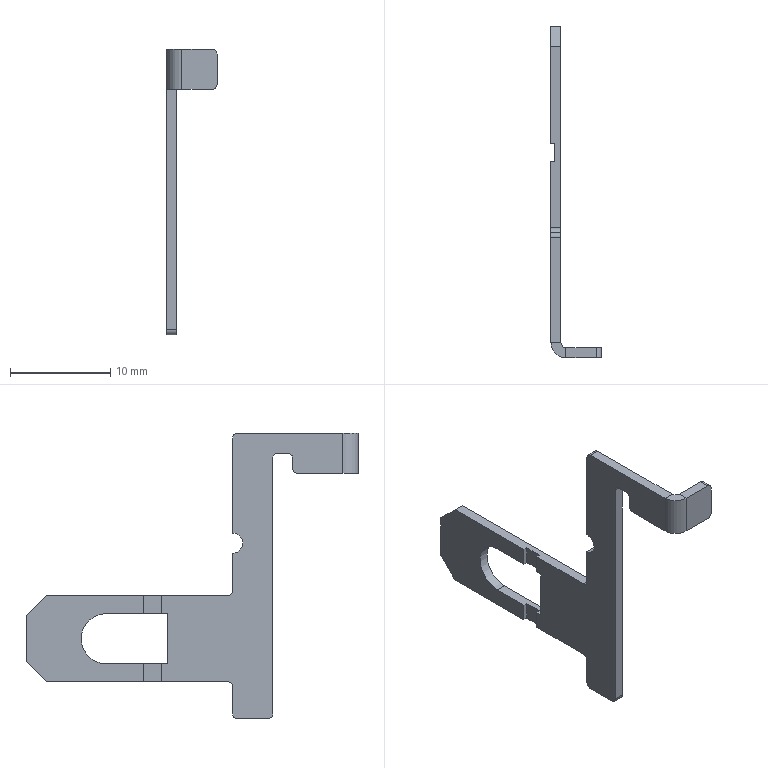Part | SolidWorks | features ICE 6, FlatPattern 2, Chamfer 1, Fillet 1, MirrorSolid 1, SMBaseFlange 1, SheetMetal 1 | 1 solid | 47 faces | box 5 x 33.1 x 28.5 mm | volume 286.856 mm3 | plane 33 | cylinder 14 | commonest cylinder face diameters 1 x11 2 x1 3 x1 5 x1
STEP:
#1=CARTESIAN_POINT('',(-4.,12.5,67.02));
#2=VERTEX_POINT('',#1);
#3=CARTESIAN_POINT('',(-5.,12.5,67.02));
#4=VERTEX_POINT('',#3);
#5=CARTESIAN_POINT('',(0.,12.5,67.02));
#6=DIRECTION('',(-1.,0.,0.));
#7=VECTOR('',#6,1000.);
#8=LINE('',#5,#7);
#9=EDGE_CURVE('',#2,#4,#8,.T.);
#10=ORIENTED_EDGE('',*,*,#9,.T.);
#11=CARTESIAN_POINT('',(-5.,12.5,76.5));
#12=VERTEX_POINT('',#11);
#13=CARTESIAN_POINT('',(-5.,12.5,73.));
#14=DIRECTION('',(0.,0.,1.));
#15=VECTOR('',#14,1000.);
#16=LINE('',#13,#15);
#17=EDGE_CURVE('',#4,#12,#16,.T.);
#18=ORIENTED_EDGE('',*,*,#17,.T.);
#19=CARTESIAN_POINT('',(-4.,12.5,76.5));
#20=VERTEX_POINT('',#19);
#21=CARTESIAN_POINT('',(-5.,12.5,76.5));
#22=DIRECTION('',(-1.,0.,0.));
#23=VECTOR('',#22,1000.);
#24=LINE('',#21,#23);
#25=EDGE_CURVE('',#20,#12,#24,.T.);
#26=ORIENTED_EDGE('',*,*,#25,.F.);
#27=CARTESIAN_POINT('',(-4.,12.5,73.));
#28=DIRECTION('',(0.,0.,1.));
#29=VECTOR('',#28,1000.);
#30=LINE('',#27,#29);
#31=EDGE_CURVE('',#2,#20,#30,.T.);
#32=ORIENTED_EDGE('',*,*,#31,.F.);
#33=EDGE_LOOP('',(#10,#18,#26,#32));
#34=FACE_OUTER_BOUND('',#33,.T.);
#35=CARTESIAN_POINT('',(-5.,12.5,73.));
#36=DIRECTION('',(0.,1.,0.));
#37=DIRECTION('',(0.,0.,-1.));
#38=AXIS2_PLACEMENT_3D('',#35,#36,#37);
#39=PLANE('',#38);
#40=ADVANCED_FACE('',(#34),#39,.T.);
#41=CARTESIAN_POINT('',(-5.,21.4,54.));
#42=VERTEX_POINT('',#41);
#43=CARTESIAN_POINT('',(-5.,21.4,52.2));
#44=VERTEX_POINT('',#43);
#45=CARTESIAN_POINT('',(-5.,21.4,77.));
#46=DIRECTION('',(0.,0.,-1.));
#47=VECTOR('',#46,1000.);
#48=LINE('',#45,#47);
#49=EDGE_CURVE('',#42,#44,#48,.T.);
#50=ORIENTED_EDGE('',*,*,#49,.T.);
#51=CARTESIAN_POINT('',(-4.6,21.4,52.2));
#52=VERTEX_POINT('',#51);
#53=CARTESIAN_POINT('',(-5.,21.4,52.2));
#54=DIRECTION('',(-1.,0.,0.));
#55=VECTOR('',#54,1000.);
#56=LINE('',#53,#55);
#57=EDGE_CURVE('',#52,#44,#56,.T.);
#58=ORIENTED_EDGE('',*,*,#57,.F.);
#59=CARTESIAN_POINT('',(-4.6,21.4,54.));
#60=VERTEX_POINT('',#59);
#61=CARTESIAN_POINT('',(-4.6,21.4,77.));
#62=DIRECTION('',(0.,0.,-1.));
#63=VECTOR('',#62,1000.);
#64=LINE('',#61,#63);
#65=EDGE_CURVE('',#60,#52,#64,.T.);
#66=ORIENTED_EDGE('',*,*,#65,.F.);
#67=CARTESIAN_POINT('',(-5.,21.4,54.));
#68=DIRECTION('',(1.,0.,0.));
#69=VECTOR('',#68,1000.);
#70=LINE('',#67,#69);
#71=EDGE_CURVE('',#42,#60,#70,.T.);
#72=ORIENTED_EDGE('',*,*,#71,.F.);
#73=EDGE_LOOP('',(#50,#58,#66,#72));
#74=FACE_OUTER_BOUND('',#73,.T.);
#75=CARTESIAN_POINT('',(-5.,21.4,77.));
#76=DIRECTION('',(0.,1.,0.));
#77=DIRECTION('',(-1.,0.,0.));
#78=AXIS2_PLACEMENT_3D('',#75,#76,#77);
#79=PLANE('',#78);
#80=ADVANCED_FACE('',(#74),#79,.F.);
#81=ORIENTED_EDGE('',*,*,#65,.T.);
#82=CARTESIAN_POINT('',(-4.6,19.6,52.2));
#83=VERTEX_POINT('',#82);
#84=CARTESIAN_POINT('',(-4.6,21.4,52.2));
#85=DIRECTION('',(0.,1.,0.));
#86=VECTOR('',#85,1000.);
#87=LINE('',#84,#86);
#88=EDGE_CURVE('',#83,#52,#87,.T.);
#89=ORIENTED_EDGE('',*,*,#88,.F.);
#90=CARTESIAN_POINT('',(-4.6,19.6,54.));
#91=VERTEX_POINT('',#90);
#92=CARTESIAN_POINT('',(-4.6,19.6,77.));
#93=DIRECTION('',(0.,0.,-1.));
#94=VECTOR('',#93,1000.);
#95=LINE('',#92,#94);
#96=EDGE_CURVE('',#91,#83,#95,.T.);
#97=ORIENTED_EDGE('',*,*,#96,.F.);
#98=CARTESIAN_POINT('',(-4.6,21.4,54.));
#99=DIRECTION('',(0.,-1.,0.));
#100=VECTOR('',#99,1000.);
#101=LINE('',#98,#100);
#102=EDGE_CURVE('',#60,#91,#101,.T.);
#103=ORIENTED_EDGE('',*,*,#102,.F.);
#104=EDGE_LOOP('',(#81,#89,#97,#103));
#105=FACE_OUTER_BOUND('',#104,.T.);
#106=CARTESIAN_POINT('',(-4.6,21.4,77.));
#107=DIRECTION('',(1.,0.,0.));
#108=DIRECTION('',(0.,1.,0.));
#109=AXIS2_PLACEMENT_3D('',#106,#107,#108);
#110=PLANE('',#109);
#111=ADVANCED_FACE('',(#105),#110,.F.);
#112=ORIENTED_EDGE('',*,*,#96,.T.);
#113=CARTESIAN_POINT('',(-5.,19.6,52.2));
#114=VERTEX_POINT('',#113);
#115=CARTESIAN_POINT('',(-5.,19.6,52.2));
#116=DIRECTION('',(1.,0.,0.));
#117=VECTOR('',#116,1000.);
#118=LINE('',#115,#117);
#119=EDGE_CURVE('',#114,#83,#118,.T.);
#120=ORIENTED_EDGE('',*,*,#119,.F.);
#121=CARTESIAN_POINT('',(-5.,19.6,54.));
#122=VERTEX_POINT('',#121);
#123=CARTESIAN_POINT('',(-5.,19.6,77.));
#124=DIRECTION('',(0.,0.,-1.));
#125=VECTOR('',#124,1000.);
#126=LINE('',#123,#125);
#127=EDGE_CURVE('',#122,#114,#126,.T.);
#128=ORIENTED_EDGE('',*,*,#127,.F.);
#129=CARTESIAN_POINT('',(-5.,19.6,54.));
#130=DIRECTION('',(-1.,0.,0.));
#131=VECTOR('',#130,1000.);
#132=LINE('',#129,#131);
#133=EDGE_CURVE('',#91,#122,#132,.T.);
#134=ORIENTED_EDGE('',*,*,#133,.F.);
#135=EDGE_LOOP('',(#112,#120,#128,#134));
#136=FACE_OUTER_BOUND('',#135,.T.);
#137=CARTESIAN_POINT('',(-5.,19.6,77.));
#138=DIRECTION('',(0.,-1.,0.));
#139=DIRECTION('',(0.,0.,1.));
#140=AXIS2_PLACEMENT_3D('',#137,#138,#139);
#141=PLANE('',#140);
#142=ADVANCED_FACE('',(#136),#141,.F.);
#143=CARTESIAN_POINT('',(-5.,31.1,52.2));
#144=VERTEX_POINT('',#143);
#145=CARTESIAN_POINT('',(-5.,12.5,52.2));
#146=DIRECTION('',(0.,1.,0.));
#147=VECTOR('',#146,1000.);
#148=LINE('',#145,#147);
#149=EDGE_CURVE('',#44,#144,#148,.T.);
#150=ORIENTED_EDGE('',*,*,#149,.F.);
#151=ORIENTED_EDGE('',*,*,#49,.F.);
#152=CARTESIAN_POINT('',(-5.,25.1,54.));
#153=VERTEX_POINT('',#152);
#154=CARTESIAN_POINT('',(-5.,25.1,54.));
#155=DIRECTION('',(0.,1.,0.));
#156=VECTOR('',#155,1000.);
#157=LINE('',#154,#156);
#158=EDGE_CURVE('',#42,#153,#157,.T.);
#159=ORIENTED_EDGE('',*,*,#158,.T.);
#160=CARTESIAN_POINT('',(-5.,25.1,59.));
#161=VERTEX_POINT('',#160);
#162=CARTESIAN_POINT('',(-5.,25.1,56.5));
#163=DIRECTION('',(1.,0.,0.));
#164=DIRECTION('',(0.,0.,-1.));
#165=AXIS2_PLACEMENT_3D('',#162,#163,#164);
#166=CIRCLE('',#165,2.5);
#167=EDGE_CURVE('',#153,#161,#166,.T.);
#168=ORIENTED_EDGE('',*,*,#167,.T.);
#169=CARTESIAN_POINT('',(-5.,21.4,59.));
#170=VERTEX_POINT('',#169);
#171=CARTESIAN_POINT('',(-5.,25.1,59.));
#172=DIRECTION('',(0.,-1.,0.));
#173=VECTOR('',#172,1000.);
#174=LINE('',#171,#173);
#175=EDGE_CURVE('',#161,#170,#174,.T.);
#176=ORIENTED_EDGE('',*,*,#175,.T.);
#177=CARTESIAN_POINT('',(-5.,21.4,60.8));
#178=VERTEX_POINT('',#177);
#179=CARTESIAN_POINT('',(-5.,21.4,77.));
#180=DIRECTION('',(0.,0.,-1.));
#181=VECTOR('',#180,1000.);
#182=LINE('',#179,#181);
#183=EDGE_CURVE('',#178,#170,#182,.T.);
#184=ORIENTED_EDGE('',*,*,#183,.F.);
#185=CARTESIAN_POINT('',(-5.,31.1,60.8));
#186=VERTEX_POINT('',#185);
#187=CARTESIAN_POINT('',(-5.,12.5,60.8));
#188=DIRECTION('',(0.,-1.,0.));
#189=VECTOR('',#188,1000.);
#190=LINE('',#187,#189);
#191=EDGE_CURVE('',#186,#178,#190,.T.);
#192=ORIENTED_EDGE('',*,*,#191,.F.);
#193=CARTESIAN_POINT('',(-5.,33.1,58.8));
#194=VERTEX_POINT('',#193);
#195=CARTESIAN_POINT('',(-5.,9.45,82.45));
#196=DIRECTION('',(0.,-0.7071,0.7071));
#197=VECTOR('',#196,1000.);
#198=LINE('',#195,#197);
#199=EDGE_CURVE('',#194,#186,#198,.T.);
#200=ORIENTED_EDGE('',*,*,#199,.F.);
#201=CARTESIAN_POINT('',(-5.,33.1,54.2));
#202=VERTEX_POINT('',#201);
#203=CARTESIAN_POINT('',(-5.,33.1,60.8));
#204=DIRECTION('',(0.,0.,1.));
#205=VECTOR('',#204,1000.);
#206=LINE('',#203,#205);
#207=EDGE_CURVE('',#202,#194,#206,.T.);
#208=ORIENTED_EDGE('',*,*,#207,.F.);
#209=CARTESIAN_POINT('',(-5.,25.95,47.05));
#210=DIRECTION('',(0.,0.7071,0.7071));
#211=VECTOR('',#210,1000.);
#212=LINE('',#209,#211);
#213=EDGE_CURVE('',#144,#202,#212,.T.);
#214=ORIENTED_EDGE('',*,*,#213,.F.);
#215=EDGE_LOOP('',(#150,#151,#159,#168,#176,#184,#192,#200,#208,#214));
#216=FACE_OUTER_BOUND('',#215,.T.);
#217=CARTESIAN_POINT('',(-5.,0.,73.));
#218=DIRECTION('',(-1.,0.,0.));
#219=DIRECTION('',(0.,0.,-1.));
#220=AXIS2_PLACEMENT_3D('',#217,#218,#219);
#221=PLANE('',#220);
#222=ADVANCED_FACE('',(#216),#221,.T.);
#223=CARTESIAN_POINT('',(-5.,12.5,49.));
#224=VERTEX_POINT('',#223);
#225=CARTESIAN_POINT('',(-5.,12.5,51.7));
#226=VERTEX_POINT('',#225);
#227=CARTESIAN_POINT('',(-5.,12.5,73.));
#228=DIRECTION('',(0.,0.,1.));
#229=VECTOR('',#228,1000.);
#230=LINE('',#227,#229);
#231=EDGE_CURVE('',#224,#226,#230,.T.);
#232=ORIENTED_EDGE('',*,*,#231,.T.);
#233=CARTESIAN_POINT('',(-4.,12.5,51.7));
#234=VERTEX_POINT('',#233);
#235=CARTESIAN_POINT('',(-5.,12.5,51.7));
#236=DIRECTION('',(-1.,0.,0.));
#237=VECTOR('',#236,1000.);
#238=LINE('',#235,#237);
#239=EDGE_CURVE('',#234,#226,#238,.T.);
#240=ORIENTED_EDGE('',*,*,#239,.F.);
#241=CARTESIAN_POINT('',(-4.,12.5,49.));
#242=VERTEX_POINT('',#241);
#243=CARTESIAN_POINT('',(-4.,12.5,73.));
#244=DIRECTION('',(0.,0.,1.));
#245=VECTOR('',#244,1000.);
#246=LINE('',#243,#245);
#247=EDGE_CURVE('',#242,#234,#246,.T.);
#248=ORIENTED_EDGE('',*,*,#247,.F.);
#249=CARTESIAN_POINT('',(-5.,12.5,49.));
#250=DIRECTION('',(1.,0.,0.));
#251=VECTOR('',#250,1000.);
#252=LINE('',#249,#251);
#253=EDGE_CURVE('',#224,#242,#252,.T.);
#254=ORIENTED_EDGE('',*,*,#253,.F.);
#255=EDGE_LOOP('',(#232,#240,#248,#254));
#256=FACE_OUTER_BOUND('',#255,.T.);
#257=CARTESIAN_POINT('',(-5.,12.5,73.));
#258=DIRECTION('',(0.,1.,0.));
#259=DIRECTION('',(0.,0.,-1.));
#260=AXIS2_PLACEMENT_3D('',#257,#258,#259);
#261=PLANE('',#260);
#262=ADVANCED_FACE('',(#256),#261,.T.);
#263=CARTESIAN_POINT('',(-4.,1.5,73.));
#264=VERTEX_POINT('',#263);
#265=CARTESIAN_POINT('',(-4.,6.,73.));
#266=VERTEX_POINT('',#265);
#267=CARTESIAN_POINT('',(-4.,0.,73.));
#268=DIRECTION('',(0.,1.,0.));
#269=VECTOR('',#268,1000.);
#270=LINE('',#267,#269);
#271=EDGE_CURVE('',#264,#266,#270,.T.);
#272=ORIENTED_EDGE('',*,*,#271,.F.);
#273=CARTESIAN_POINT('',(-5.,1.5,73.));
#274=VERTEX_POINT('',#273);
#275=CARTESIAN_POINT('',(-5.,1.5,73.));
#276=DIRECTION('',(1.,0.,0.));
#277=VECTOR('',#276,1000.);
#278=LINE('',#275,#277);
#279=EDGE_CURVE('',#274,#264,#278,.T.);
#280=ORIENTED_EDGE('',*,*,#279,.F.);
#281=CARTESIAN_POINT('',(-5.,6.,73.));
#282=VERTEX_POINT('',#281);
#283=CARTESIAN_POINT('',(-5.,0.,73.));
#284=DIRECTION('',(0.,1.,0.));
#285=VECTOR('',#284,1000.);
#286=LINE('',#283,#285);
#287=EDGE_CURVE('',#274,#282,#286,.T.);
#288=ORIENTED_EDGE('',*,*,#287,.T.);
#289=CARTESIAN_POINT('',(-5.,6.,73.));
#290=DIRECTION('',(-1.,0.,0.));
#291=VECTOR('',#290,1000.);
#292=LINE('',#289,#291);
#293=EDGE_CURVE('',#266,#282,#292,.T.);
#294=ORIENTED_EDGE('',*,*,#293,.F.);
#295=EDGE_LOOP('',(#272,#280,#288,#294));
#296=FACE_OUTER_BOUND('',#295,.T.);
#297=CARTESIAN_POINT('',(-3.5,1.,73.));
#298=DIRECTION('',(0.,0.,-1.));
#299=DIRECTION('',(1.,0.,0.));
#300=AXIS2_PLACEMENT_3D('',#297,#298,#299);
#301=PLANE('',#300);
#302=ADVANCED_FACE('',(#296),#301,.T.);
#303=ORIENTED_EDGE('',*,*,#279,.T.);
#304=CARTESIAN_POINT('',(-3.5,1.,73.));
#305=VERTEX_POINT('',#304);
#306=CARTESIAN_POINT('',(-3.5,1.5,73.));
#307=DIRECTION('',(0.,0.,-1.));
#308=DIRECTION('',(1.,0.,0.));
#309=AXIS2_PLACEMENT_3D('',#306,#307,#308);
#310=CIRCLE('',#309,0.5);
#311=EDGE_CURVE('',#305,#264,#310,.T.);
#312=ORIENTED_EDGE('',*,*,#311,.F.);
#313=CARTESIAN_POINT('',(-3.5,0.,73.));
#314=VERTEX_POINT('',#313);
#315=CARTESIAN_POINT('',(-3.5,1.,73.));
#316=DIRECTION('',(0.,-1.,0.));
#317=VECTOR('',#316,1000.);
#318=LINE('',#315,#317);
#319=EDGE_CURVE('',#305,#314,#318,.T.);
#320=ORIENTED_EDGE('',*,*,#319,.T.);
#321=CARTESIAN_POINT('',(-3.5,1.5,73.));
#322=DIRECTION('',(0.,0.,-1.));
#323=DIRECTION('',(1.,0.,0.));
#324=AXIS2_PLACEMENT_3D('',#321,#322,#323);
#325=CIRCLE('',#324,1.5);
#326=EDGE_CURVE('',#314,#274,#325,.T.);
#327=ORIENTED_EDGE('',*,*,#326,.T.);
#328=EDGE_LOOP('',(#303,#312,#320,#327));
#329=FACE_OUTER_BOUND('',#328,.T.);
#330=CARTESIAN_POINT('',(-5.,1.5,73.));
#331=DIRECTION('',(0.,0.,-1.));
#332=DIRECTION('',(1.,0.,0.));
#333=AXIS2_PLACEMENT_3D('',#330,#331,#332);
#334=PLANE('',#333);
#335=ADVANCED_FACE('',(#329),#334,.T.);
#336=CARTESIAN_POINT('',(-3.5,0.,77.));
#337=VERTEX_POINT('',#336);
#338=CARTESIAN_POINT('',(-3.5,1.,77.));
#339=VERTEX_POINT('',#338);
#340=CARTESIAN_POINT('',(-3.5,0.,77.));
#341=DIRECTION('',(0.,1.,0.));
#342=VECTOR('',#341,1000.);
#343=LINE('',#340,#342);
#344=EDGE_CURVE('',#337,#339,#343,.T.);
#345=ORIENTED_EDGE('',*,*,#344,.T.);
#346=CARTESIAN_POINT('',(-4.,1.5,77.));
#347=VERTEX_POINT('',#346);
#348=CARTESIAN_POINT('',(-3.5,1.5,77.));
#349=DIRECTION('',(0.,0.,-1.));
#350=DIRECTION('',(1.,0.,0.));
#351=AXIS2_PLACEMENT_3D('',#348,#349,#350);
#352=CIRCLE('',#351,0.5);
#353=EDGE_CURVE('',#339,#347,#352,.T.);
#354=ORIENTED_EDGE('',*,*,#353,.T.);
#355=CARTESIAN_POINT('',(-5.,1.5,77.));
#356=VERTEX_POINT('',#355);
#357=CARTESIAN_POINT('',(-4.,1.5,77.));
#358=DIRECTION('',(-1.,0.,0.));
#359=VECTOR('',#358,1000.);
#360=LINE('',#357,#359);
#361=EDGE_CURVE('',#347,#356,#360,.T.);
#362=ORIENTED_EDGE('',*,*,#361,.T.);
#363=CARTESIAN_POINT('',(-3.5,1.5,77.));
#364=DIRECTION('',(0.,0.,-1.));
#365=DIRECTION('',(1.,0.,0.));
#366=AXIS2_PLACEMENT_3D('',#363,#364,#365);
#367=CIRCLE('',#366,1.5);
#368=EDGE_CURVE('',#337,#356,#367,.T.);
#369=ORIENTED_EDGE('',*,*,#368,.F.);
#370=EDGE_LOOP('',(#345,#354,#362,#369));
#371=FACE_OUTER_BOUND('',#370,.T.);
#372=CARTESIAN_POINT('',(-3.5,0.,77.));
#373=DIRECTION('',(0.,0.,1.));
#374=DIRECTION('',(-1.,0.,0.));
#375=AXIS2_PLACEMENT_3D('',#372,#373,#374);
#376=PLANE('',#375);
#377=ADVANCED_FACE('',(#371),#376,.T.);
#378=CARTESIAN_POINT('',(-0.5,1.,77.));
#379=VERTEX_POINT('',#378);
#380=CARTESIAN_POINT('',(0.,1.,77.));
#381=DIRECTION('',(-1.,0.,0.));
#382=VECTOR('',#381,1000.);
#383=LINE('',#380,#382);
#384=EDGE_CURVE('',#379,#339,#383,.T.);
#385=ORIENTED_EDGE('',*,*,#384,.T.);
#386=ORIENTED_EDGE('',*,*,#344,.F.);
#387=CARTESIAN_POINT('',(-0.5,0.,77.));
#388=VERTEX_POINT('',#387);
#389=CARTESIAN_POINT('',(0.,0.,77.));
#390=DIRECTION('',(-1.,0.,0.));
#391=VECTOR('',#390,1000.);
#392=LINE('',#389,#391);
#393=EDGE_CURVE('',#388,#337,#392,.T.);
#394=ORIENTED_EDGE('',*,*,#393,.F.);
#395=CARTESIAN_POINT('',(-0.5,1.5,77.));
#396=DIRECTION('',(0.,-1.,0.));
#397=VECTOR('',#396,1000.);
#398=LINE('',#395,#397);
#399=EDGE_CURVE('',#379,#388,#398,.T.);
#400=ORIENTED_EDGE('',*,*,#399,.F.);
#401=EDGE_LOOP('',(#385,#386,#394,#400));
#402=FACE_OUTER_BOUND('',#401,.T.);
#403=CARTESIAN_POINT('',(-4.,1.5,77.));
#404=DIRECTION('',(0.,0.,1.));
#405=DIRECTION('',(-1.,0.,0.));
#406=AXIS2_PLACEMENT_3D('',#403,#404,#405);
#407=PLANE('',#406);
#408=ADVANCED_FACE('',(#402),#407,.T.);
#409=CARTESIAN_POINT('',(-4.,19.,54.));
#410=VERTEX_POINT('',#409);
#411=CARTESIAN_POINT('',(-4.,25.1,54.));
#412=VERTEX_POINT('',#411);
#413=CARTESIAN_POINT('',(-4.,0.,54.));
#414=DIRECTION('',(0.,1.,0.));
#415=VECTOR('',#414,1000.);
#416=LINE('',#413,#415);
#417=EDGE_CURVE('',#410,#412,#416,.T.);
#418=ORIENTED_EDGE('',*,*,#417,.F.);
#419=CARTESIAN_POINT('',(-4.,19.,59.));
#420=VERTEX_POINT('',#419);
#421=CARTESIAN_POINT('',(-4.,19.,73.));
#422=DIRECTION('',(0.,0.,-1.));
#423=VECTOR('',#422,1000.);
#424=LINE('',#421,#423);
#425=EDGE_CURVE('',#420,#410,#424,.T.);
#426=ORIENTED_EDGE('',*,*,#425,.F.);
#427=CARTESIAN_POINT('',(-4.,25.1,59.));
#428=VERTEX_POINT('',#427);
#429=CARTESIAN_POINT('',(-4.,0.,59.));
#430=DIRECTION('',(0.,-1.,0.));
#431=VECTOR('',#430,1000.);
#432=LINE('',#429,#431);
#433=EDGE_CURVE('',#428,#420,#432,.T.);
#434=ORIENTED_EDGE('',*,*,#433,.F.);
#435=CARTESIAN_POINT('',(-4.,25.1,56.5));
#436=DIRECTION('',(1.,0.,0.));
#437=DIRECTION('',(0.,0.,-1.));
#438=AXIS2_PLACEMENT_3D('',#435,#436,#437);
#439=CIRCLE('',#438,2.5);
#440=EDGE_CURVE('',#412,#428,#439,.T.);
#441=ORIENTED_EDGE('',*,*,#440,.F.);
#442=EDGE_LOOP('',(#418,#426,#434,#441));
#443=FACE_BOUND('',#442,.T.);
#444=ORIENTED_EDGE('',*,*,#31,.T.);
#445=CARTESIAN_POINT('',(-4.,12.,77.));
#446=VERTEX_POINT('',#445);
#447=CARTESIAN_POINT('',(-4.,12.,76.5));
#448=DIRECTION('',(-1.,0.,0.));
#449=DIRECTION('',(0.,0.,-1.));
#450=AXIS2_PLACEMENT_3D('',#447,#448,#449);
#451=CIRCLE('',#450,0.5);
#452=EDGE_CURVE('',#446,#20,#451,.T.);
#453=ORIENTED_EDGE('',*,*,#452,.F.);
#454=CARTESIAN_POINT('',(-4.,0.,77.));
#455=DIRECTION('',(0.,1.,0.));
#456=VECTOR('',#455,1000.);
#457=LINE('',#454,#456);
#458=EDGE_CURVE('',#347,#446,#457,.T.);
#459=ORIENTED_EDGE('',*,*,#458,.F.);
#460=CARTESIAN_POINT('',(-4.,1.5,73.));
#461=DIRECTION('',(0.,0.,1.));
#462=VECTOR('',#461,1000.);
#463=LINE('',#460,#462);
#464=EDGE_CURVE('',#264,#347,#463,.T.);
#465=ORIENTED_EDGE('',*,*,#464,.F.);
#466=ORIENTED_EDGE('',*,*,#271,.T.);
#467=CARTESIAN_POINT('',(-4.,6.5,73.5));
#468=VERTEX_POINT('',#467);
#469=CARTESIAN_POINT('',(-4.,6.,73.5));
#470=DIRECTION('',(-1.,0.,0.));
#471=DIRECTION('',(0.,0.,-1.));
#472=AXIS2_PLACEMENT_3D('',#469,#470,#471);
#473=CIRCLE('',#472,0.5);
#474=EDGE_CURVE('',#468,#266,#473,.T.);
#475=ORIENTED_EDGE('',*,*,#474,.F.);
#476=CARTESIAN_POINT('',(-4.,6.5,74.5));
#477=VERTEX_POINT('',#476);
#478=CARTESIAN_POINT('',(-4.,6.5,73.));
#479=DIRECTION('',(0.,0.,-1.));
#480=VECTOR('',#479,1000.);
#481=LINE('',#478,#480);
#482=EDGE_CURVE('',#477,#468,#481,.T.);
#483=ORIENTED_EDGE('',*,*,#482,.F.);
#484=CARTESIAN_POINT('',(-4.,7.,75.));
#485=VERTEX_POINT('',#484);
#486=CARTESIAN_POINT('',(-4.,7.,74.5));
#487=DIRECTION('',(1.,0.,0.));
#488=DIRECTION('',(0.,0.,-1.));
#489=AXIS2_PLACEMENT_3D('',#486,#487,#488);
#490=CIRCLE('',#489,0.5);
#491=EDGE_CURVE('',#485,#477,#490,.T.);
#492=ORIENTED_EDGE('',*,*,#491,.F.);
#493=CARTESIAN_POINT('',(-4.,8.,75.));
#494=VERTEX_POINT('',#493);
#495=CARTESIAN_POINT('',(-4.,0.,75.));
#496=DIRECTION('',(0.,-1.,0.));
#497=VECTOR('',#496,1000.);
#498=LINE('',#495,#497);
#499=EDGE_CURVE('',#494,#485,#498,.T.);
#500=ORIENTED_EDGE('',*,*,#499,.F.);
#501=CARTESIAN_POINT('',(-4.,8.5,74.5));
#502=VERTEX_POINT('',#501);
#503=CARTESIAN_POINT('',(-4.,8.,74.5));
#504=DIRECTION('',(1.,0.,0.));
#505=DIRECTION('',(0.,0.,-1.));
#506=AXIS2_PLACEMENT_3D('',#503,#504,#505);
#507=CIRCLE('',#506,0.5);
#508=EDGE_CURVE('',#502,#494,#507,.T.);
#509=ORIENTED_EDGE('',*,*,#508,.F.);
#510=CARTESIAN_POINT('',(-4.,8.5,49.));
#511=VERTEX_POINT('',#510);
#512=CARTESIAN_POINT('',(-4.,8.5,73.));
#513=DIRECTION('',(0.,0.,1.));
#514=VECTOR('',#513,1000.);
#515=LINE('',#512,#514);
#516=EDGE_CURVE('',#511,#502,#515,.T.);
#517=ORIENTED_EDGE('',*,*,#516,.F.);
#518=CARTESIAN_POINT('',(-4.,9.,48.5));
#519=VERTEX_POINT('',#518);
#520=CARTESIAN_POINT('',(-4.,9.,49.));
#521=DIRECTION('',(-1.,0.,0.));
#522=DIRECTION('',(0.,0.,-1.));
#523=AXIS2_PLACEMENT_3D('',#520,#521,#522);
#524=CIRCLE('',#523,0.5);
#525=EDGE_CURVE('',#519,#511,#524,.T.);
#526=ORIENTED_EDGE('',*,*,#525,.F.);
#527=CARTESIAN_POINT('',(-4.,12.,48.5));
#528=VERTEX_POINT('',#527);
#529=CARTESIAN_POINT('',(-4.,8.5,48.5));
#530=DIRECTION('',(0.,1.,0.));
#531=VECTOR('',#530,1000.);
#532=LINE('',#529,#531);
#533=EDGE_CURVE('',#519,#528,#532,.T.);
#534=ORIENTED_EDGE('',*,*,#533,.T.);
#535=CARTESIAN_POINT('',(-4.,12.,49.));
#536=DIRECTION('',(-1.,0.,0.));
#537=DIRECTION('',(0.,0.,-1.));
#538=AXIS2_PLACEMENT_3D('',#535,#536,#537);
#539=CIRCLE('',#538,0.5);
#540=EDGE_CURVE('',#242,#528,#539,.T.);
#541=ORIENTED_EDGE('',*,*,#540,.F.);
#542=ORIENTED_EDGE('',*,*,#247,.T.);
#543=CARTESIAN_POINT('',(-4.,13.,52.2));
#544=VERTEX_POINT('',#543);
#545=CARTESIAN_POINT('',(-4.,13.,51.7));
#546=DIRECTION('',(1.,0.,0.));
#547=DIRECTION('',(0.,0.,-1.));
#548=AXIS2_PLACEMENT_3D('',#545,#546,#547);
#549=CIRCLE('',#548,0.5);
#550=EDGE_CURVE('',#544,#234,#549,.T.);
#551=ORIENTED_EDGE('',*,*,#550,.F.);
#552=CARTESIAN_POINT('',(-4.,31.1,52.2));
#553=VERTEX_POINT('',#552);
#554=CARTESIAN_POINT('',(-4.,12.5,52.2));
#555=DIRECTION('',(0.,-1.,0.));
#556=VECTOR('',#555,1000.);
#557=LINE('',#554,#556);
#558=EDGE_CURVE('',#553,#544,#557,.T.);
#559=ORIENTED_EDGE('',*,*,#558,.F.);
#560=CARTESIAN_POINT('',(-4.,33.1,54.2));
#561=VERTEX_POINT('',#560);
#562=CARTESIAN_POINT('',(-4.,31.1,52.2));
#563=DIRECTION('',(0.,-0.7071,-0.7071));
#564=VECTOR('',#563,1000.);
#565=LINE('',#562,#564);
#566=EDGE_CURVE('',#561,#553,#565,.T.);
#567=ORIENTED_EDGE('',*,*,#566,.F.);
#568=CARTESIAN_POINT('',(-4.,33.1,58.8));
#569=VERTEX_POINT('',#568);
#570=CARTESIAN_POINT('',(-4.,33.1,60.8));
#571=DIRECTION('',(0.,0.,-1.));
#572=VECTOR('',#571,1000.);
#573=LINE('',#570,#572);
#574=EDGE_CURVE('',#569,#561,#573,.T.);
#575=ORIENTED_EDGE('',*,*,#574,.F.);
#576=CARTESIAN_POINT('',(-4.,31.1,60.8));
#577=VERTEX_POINT('',#576);
#578=CARTESIAN_POINT('',(-4.,33.1,58.8));
#579=DIRECTION('',(0.,0.7071,-0.7071));
#580=VECTOR('',#579,1000.);
#581=LINE('',#578,#580);
#582=EDGE_CURVE('',#577,#569,#581,.T.);
#583=ORIENTED_EDGE('',*,*,#582,.F.);
#584=CARTESIAN_POINT('',(-4.,13.,60.8));
#585=VERTEX_POINT('',#584);
#586=CARTESIAN_POINT('',(-4.,12.5,60.8));
#587=DIRECTION('',(0.,1.,0.));
#588=VECTOR('',#587,1000.);
#589=LINE('',#586,#588);
#590=EDGE_CURVE('',#585,#577,#589,.T.);
#591=ORIENTED_EDGE('',*,*,#590,.F.);
#592=CARTESIAN_POINT('',(-4.,12.5,61.3));
#593=VERTEX_POINT('',#592);
#594=CARTESIAN_POINT('',(-4.,13.,61.3));
#595=DIRECTION('',(1.,0.,0.));
#596=DIRECTION('',(0.,0.,-1.));
#597=AXIS2_PLACEMENT_3D('',#594,#595,#596);
#598=CIRCLE('',#597,0.5);
#599=EDGE_CURVE('',#593,#585,#598,.T.);
#600=ORIENTED_EDGE('',*,*,#599,.F.);
#601=CARTESIAN_POINT('',(-4.,12.5,65.02));
#602=VERTEX_POINT('',#601);
#603=CARTESIAN_POINT('',(-4.,12.5,73.));
#604=DIRECTION('',(0.,0.,1.));
#605=VECTOR('',#604,1000.);
#606=LINE('',#603,#605);
#607=EDGE_CURVE('',#593,#602,#606,.T.);
#608=ORIENTED_EDGE('',*,*,#607,.T.);
#609=CARTESIAN_POINT('',(-4.,12.5,66.02));
#610=DIRECTION('',(1.,0.,0.));
#611=DIRECTION('',(0.,0.,-1.));
#612=AXIS2_PLACEMENT_3D('',#609,#610,#611);
#613=CIRCLE('',#612,1.);
#614=EDGE_CURVE('',#2,#602,#613,.T.);
#615=ORIENTED_EDGE('',*,*,#614,.F.);
#616=EDGE_LOOP('',(#444,#453,#459,#465,#466,#475,#483,#492,#500,#509,#517,#526,#534,#541,#542,#551,#559,#567,#575,#583,#591,#600,#608,#615));
#617=FACE_OUTER_BOUND('',#616,.T.);
#618=CARTESIAN_POINT('',(-4.,0.,73.));
#619=DIRECTION('',(-1.,0.,0.));
#620=DIRECTION('',(0.,0.,-1.));
#621=AXIS2_PLACEMENT_3D('',#618,#619,#620);
#622=PLANE('',#621);
#623=ADVANCED_FACE('',(#443,#617),#622,.F.);
#624=CARTESIAN_POINT('',(-5.,12.5,65.02));
#625=VERTEX_POINT('',#624);
#626=CARTESIAN_POINT('',(0.,12.5,65.02));
#627=DIRECTION('',(1.,0.,0.));
#628=VECTOR('',#627,1000.);
#629=LINE('',#626,#628);
#630=EDGE_CURVE('',#625,#602,#629,.T.);
#631=ORIENTED_EDGE('',*,*,#630,.T.);
#632=ORIENTED_EDGE('',*,*,#607,.F.);
#633=CARTESIAN_POINT('',(-5.,12.5,61.3));
#634=VERTEX_POINT('',#633);
#635=CARTESIAN_POINT('',(-4.,12.5,61.3));
#636=DIRECTION('',(1.,0.,0.));
#637=VECTOR('',#636,1000.);
#638=LINE('',#635,#637);
#639=EDGE_CURVE('',#634,#593,#638,.T.);
#640=ORIENTED_EDGE('',*,*,#639,.F.);
#641=CARTESIAN_POINT('',(-5.,12.5,73.));
#642=DIRECTION('',(0.,0.,1.));
#643=VECTOR('',#642,1000.);
#644=LINE('',#641,#643);
#645=EDGE_CURVE('',#634,#625,#644,.T.);
#646=ORIENTED_EDGE('',*,*,#645,.T.);
#647=EDGE_LOOP('',(#631,#632,#640,#646));
#648=FACE_OUTER_BOUND('',#647,.T.);
#649=CARTESIAN_POINT('',(-5.,12.5,73.));
#650=DIRECTION('',(0.,1.,0.));
#651=DIRECTION('',(0.,0.,-1.));
#652=AXIS2_PLACEMENT_3D('',#649,#650,#651);
#653=PLANE('',#652);
#654=ADVANCED_FACE('',(#648),#653,.T.);
#655=CARTESIAN_POINT('',(-5.,12.5,66.02));
#656=DIRECTION('',(1.,0.,0.));
#657=DIRECTION('',(0.,0.,-1.));
#658=AXIS2_PLACEMENT_3D('',#655,#656,#657);
#659=CIRCLE('',#658,1.);
#660=EDGE_CURVE('',#4,#625,#659,.T.);
#661=ORIENTED_EDGE('',*,*,#660,.T.);
#662=ORIENTED_EDGE('',*,*,#645,.F.);
#663=CARTESIAN_POINT('',(-5.,13.,60.8));
#664=VERTEX_POINT('',#663);
#665=CARTESIAN_POINT('',(-5.,13.,61.3));
#666=DIRECTION('',(-1.,0.,0.));
#667=DIRECTION('',(0.,0.,-1.));
#668=AXIS2_PLACEMENT_3D('',#665,#666,#667);
#669=CIRCLE('',#668,0.5);
#670=EDGE_CURVE('',#664,#634,#669,.T.);
#671=ORIENTED_EDGE('',*,*,#670,.F.);
#672=CARTESIAN_POINT('',(-5.,19.6,60.8));
#673=VERTEX_POINT('',#672);
#674=CARTESIAN_POINT('',(-5.,12.5,60.8));
#675=DIRECTION('',(0.,-1.,0.));
#676=VECTOR('',#675,1000.);
#677=LINE('',#674,#676);
#678=EDGE_CURVE('',#673,#664,#677,.T.);
#679=ORIENTED_EDGE('',*,*,#678,.F.);
#680=CARTESIAN_POINT('',(-5.,19.6,59.));
#681=VERTEX_POINT('',#680);
#682=CARTESIAN_POINT('',(-5.,19.6,77.));
#683=DIRECTION('',(0.,0.,-1.));
#684=VECTOR('',#683,1000.);
#685=LINE('',#682,#684);
#686=EDGE_CURVE('',#673,#681,#685,.T.);
#687=ORIENTED_EDGE('',*,*,#686,.T.);
#688=CARTESIAN_POINT('',(-5.,19.,59.));
#689=VERTEX_POINT('',#688);
#690=CARTESIAN_POINT('',(-5.,25.1,59.));
#691=DIRECTION('',(0.,-1.,0.));
#692=VECTOR('',#691,1000.);
#693=LINE('',#690,#692);
#694=EDGE_CURVE('',#681,#689,#693,.T.);
#695=ORIENTED_EDGE('',*,*,#694,.T.);
#696=CARTESIAN_POINT('',(-5.,19.,54.));
#697=VERTEX_POINT('',#696);
#698=CARTESIAN_POINT('',(-5.,19.,59.));
#699=DIRECTION('',(0.,0.,-1.));
#700=VECTOR('',#699,1000.);
#701=LINE('',#698,#700);
#702=EDGE_CURVE('',#689,#697,#701,.T.);
#703=ORIENTED_EDGE('',*,*,#702,.T.);
#704=CARTESIAN_POINT('',(-5.,25.1,54.));
#705=DIRECTION('',(0.,1.,0.));
#706=VECTOR('',#705,1000.);
#707=LINE('',#704,#706);
#708=EDGE_CURVE('',#697,#122,#707,.T.);
#709=ORIENTED_EDGE('',*,*,#708,.T.);
#710=ORIENTED_EDGE('',*,*,#127,.T.);
#711=CARTESIAN_POINT('',(-5.,13.,52.2));
#712=VERTEX_POINT('',#711);
#713=CARTESIAN_POINT('',(-5.,12.5,52.2));
#714=DIRECTION('',(0.,1.,0.));
#715=VECTOR('',#714,1000.);
#716=LINE('',#713,#715);
#717=EDGE_CURVE('',#712,#114,#716,.T.);
#718=ORIENTED_EDGE('',*,*,#717,.F.);
#719=CARTESIAN_POINT('',(-5.,13.,51.7));
#720=DIRECTION('',(-1.,0.,0.));
#721=DIRECTION('',(0.,0.,-1.));
#722=AXIS2_PLACEMENT_3D('',#719,#720,#721);
#723=CIRCLE('',#722,0.5);
#724=EDGE_CURVE('',#226,#712,#723,.T.);
#725=ORIENTED_EDGE('',*,*,#724,.F.);
#726=ORIENTED_EDGE('',*,*,#231,.F.);
#727=CARTESIAN_POINT('',(-5.,12.,48.5));
#728=VERTEX_POINT('',#727);
#729=CARTESIAN_POINT('',(-5.,12.,49.));
#730=DIRECTION('',(1.,0.,0.));
#731=DIRECTION('',(0.,0.,-1.));
#732=AXIS2_PLACEMENT_3D('',#729,#730,#731);
#733=CIRCLE('',#732,0.5);
#734=EDGE_CURVE('',#728,#224,#733,.T.);
#735=ORIENTED_EDGE('',*,*,#734,.F.);
#736=CARTESIAN_POINT('',(-5.,9.,48.5));
#737=VERTEX_POINT('',#736);
#738=CARTESIAN_POINT('',(-5.,8.5,48.5));
#739=DIRECTION('',(0.,1.,0.));
#740=VECTOR('',#739,1000.);
#741=LINE('',#738,#740);
#742=EDGE_CURVE('',#737,#728,#741,.T.);
#743=ORIENTED_EDGE('',*,*,#742,.F.);
#744=CARTESIAN_POINT('',(-5.,8.5,49.));
#745=VERTEX_POINT('',#744);
#746=CARTESIAN_POINT('',(-5.,9.,49.));
#747=DIRECTION('',(1.,0.,0.));
#748=DIRECTION('',(0.,0.,-1.));
#749=AXIS2_PLACEMENT_3D('',#746,#747,#748);
#750=CIRCLE('',#749,0.5);
#751=EDGE_CURVE('',#745,#737,#750,.T.);
#752=ORIENTED_EDGE('',*,*,#751,.F.);
#753=CARTESIAN_POINT('',(-5.,8.5,74.5));
#754=VERTEX_POINT('',#753);
#755=CARTESIAN_POINT('',(-5.,8.5,73.));
#756=DIRECTION('',(0.,0.,-1.));
#757=VECTOR('',#756,1000.);
#758=LINE('',#755,#757);
#759=EDGE_CURVE('',#754,#745,#758,.T.);
#760=ORIENTED_EDGE('',*,*,#759,.F.);
#761=CARTESIAN_POINT('',(-5.,8.,75.));
#762=VERTEX_POINT('',#761);
#763=CARTESIAN_POINT('',(-5.,8.,74.5));
#764=DIRECTION('',(-1.,0.,0.));
#765=DIRECTION('',(0.,0.,-1.));
#766=AXIS2_PLACEMENT_3D('',#763,#764,#765);
#767=CIRCLE('',#766,0.5);
#768=EDGE_CURVE('',#762,#754,#767,.T.);
#769=ORIENTED_EDGE('',*,*,#768,.F.);
#770=CARTESIAN_POINT('',(-5.,7.,75.));
#771=VERTEX_POINT('',#770);
#772=CARTESIAN_POINT('',(-5.,8.5,75.));
#773=DIRECTION('',(0.,-1.,0.));
#774=VECTOR('',#773,1000.);
#775=LINE('',#772,#774);
#776=EDGE_CURVE('',#762,#771,#775,.T.);
#777=ORIENTED_EDGE('',*,*,#776,.T.);
#778=CARTESIAN_POINT('',(-5.,6.5,74.5));
#779=VERTEX_POINT('',#778);
#780=CARTESIAN_POINT('',(-5.,7.,74.5));
#781=DIRECTION('',(-1.,0.,0.));
#782=DIRECTION('',(0.,0.,-1.));
#783=AXIS2_PLACEMENT_3D('',#780,#781,#782);
#784=CIRCLE('',#783,0.5);
#785=EDGE_CURVE('',#779,#771,#784,.T.);
#786=ORIENTED_EDGE('',*,*,#785,.F.);
#787=CARTESIAN_POINT('',(-5.,6.5,73.5));
#788=VERTEX_POINT('',#787);
#789=CARTESIAN_POINT('',(-5.,6.5,75.));
#790=DIRECTION('',(0.,0.,-1.));
#791=VECTOR('',#790,1000.);
#792=LINE('',#789,#791);
#793=EDGE_CURVE('',#779,#788,#792,.T.);
#794=ORIENTED_EDGE('',*,*,#793,.T.);
#795=CARTESIAN_POINT('',(-5.,6.,73.5));
#796=DIRECTION('',(1.,0.,0.));
#797=DIRECTION('',(0.,0.,-1.));
#798=AXIS2_PLACEMENT_3D('',#795,#796,#797);
#799=CIRCLE('',#798,0.5);
#800=EDGE_CURVE('',#282,#788,#799,.T.);
#801=ORIENTED_EDGE('',*,*,#800,.F.);
#802=ORIENTED_EDGE('',*,*,#287,.F.);
#803=CARTESIAN_POINT('',(-5.,1.5,73.));
#804=DIRECTION('',(0.,0.,1.));
#805=VECTOR('',#804,1000.);
#806=LINE('',#803,#805);
#807=EDGE_CURVE('',#274,#356,#806,.T.);
#808=ORIENTED_EDGE('',*,*,#807,.T.);
#809=CARTESIAN_POINT('',(-5.,12.,77.));
#810=VERTEX_POINT('',#809);
#811=CARTESIAN_POINT('',(-5.,0.,77.));
#812=DIRECTION('',(0.,1.,0.));
#813=VECTOR('',#812,1000.);
#814=LINE('',#811,#813);
#815=EDGE_CURVE('',#356,#810,#814,.T.);
#816=ORIENTED_EDGE('',*,*,#815,.T.);
#817=CARTESIAN_POINT('',(-5.,12.,76.5));
#818=DIRECTION('',(1.,0.,0.));
#819=DIRECTION('',(0.,0.,-1.));
#820=AXIS2_PLACEMENT_3D('',#817,#818,#819);
#821=CIRCLE('',#820,0.5);
#822=EDGE_CURVE('',#12,#810,#821,.T.);
#823=ORIENTED_EDGE('',*,*,#822,.F.);
#824=ORIENTED_EDGE('',*,*,#17,.F.);
#825=EDGE_LOOP('',(#661,#662,#671,#679,#687,#695,#703,#709,#710,#718,#725,#726,#735,#743,#752,#760,#769,#777,#786,#794,#801,#802,#808,#816,#823,#824));
#826=FACE_OUTER_BOUND('',#825,.T.);
#827=CARTESIAN_POINT('',(-5.,0.,73.));
#828=DIRECTION('',(-1.,0.,0.));
#829=DIRECTION('',(0.,0.,-1.));
#830=AXIS2_PLACEMENT_3D('',#827,#828,#829);
#831=PLANE('',#830);
#832=ADVANCED_FACE('',(#826),#831,.T.);
#833=ORIENTED_EDGE('',*,*,#368,.T.);
#834=ORIENTED_EDGE('',*,*,#807,.F.);
#835=ORIENTED_EDGE('',*,*,#326,.F.);
#836=CARTESIAN_POINT('',(-3.5,0.,73.));
#837=DIRECTION('',(0.,0.,1.));
#838=VECTOR('',#837,1000.);
#839=LINE('',#836,#838);
#840=EDGE_CURVE('',#314,#337,#839,.T.);
#841=ORIENTED_EDGE('',*,*,#840,.T.);
#842=EDGE_LOOP('',(#833,#834,#835,#841));
#843=FACE_OUTER_BOUND('',#842,.T.);
#844=CARTESIAN_POINT('',(-3.5,1.5,73.));
#845=DIRECTION('',(0.,0.,1.));
#846=DIRECTION('',(-1.,0.,0.));
#847=AXIS2_PLACEMENT_3D('',#844,#845,#846);
#848=CYLINDRICAL_SURFACE('',#847,1.5);
#849=ADVANCED_FACE('',(#843),#848,.T.);
#850=CARTESIAN_POINT('',(0.,0.,73.5));
#851=VERTEX_POINT('',#850);
#852=CARTESIAN_POINT('',(0.,0.,76.5));
#853=VERTEX_POINT('',#852);
#854=CARTESIAN_POINT('',(0.,0.,73.));
#855=DIRECTION('',(0.,0.,1.));
#856=VECTOR('',#855,1000.);
#857=LINE('',#854,#856);
#858=EDGE_CURVE('',#851,#853,#857,.T.);
#859=ORIENTED_EDGE('',*,*,#858,.T.);
#860=CARTESIAN_POINT('',(-0.5,0.,76.5));
#861=DIRECTION('',(0.,1.,0.));
#862=DIRECTION('',(0.,0.,1.));
#863=AXIS2_PLACEMENT_3D('',#860,#861,#862);
#864=CIRCLE('',#863,0.5);
#865=EDGE_CURVE('',#388,#853,#864,.T.);
#866=ORIENTED_EDGE('',*,*,#865,.F.);
#867=ORIENTED_EDGE('',*,*,#393,.T.);
#868=ORIENTED_EDGE('',*,*,#840,.F.);
#869=CARTESIAN_POINT('',(-0.5,0.,73.));
#870=VERTEX_POINT('',#869);
#871=CARTESIAN_POINT('',(0.,0.,73.));
#872=DIRECTION('',(-1.,0.,0.));
#873=VECTOR('',#872,1000.);
#874=LINE('',#871,#873);
#875=EDGE_CURVE('',#870,#314,#874,.T.);
#876=ORIENTED_EDGE('',*,*,#875,.F.);
#877=CARTESIAN_POINT('',(-0.5,0.,73.5));
#878=DIRECTION('',(0.,1.,0.));
#879=DIRECTION('',(0.,0.,1.));
#880=AXIS2_PLACEMENT_3D('',#877,#878,#879);
#881=CIRCLE('',#880,0.5);
#882=EDGE_CURVE('',#851,#870,#881,.T.);
#883=ORIENTED_EDGE('',*,*,#882,.F.);
#884=EDGE_LOOP('',(#859,#866,#867,#868,#876,#883));
#885=FACE_OUTER_BOUND('',#884,.T.);
#886=CARTESIAN_POINT('',(0.,0.,73.));
#887=DIRECTION('',(0.,-1.,0.));
#888=DIRECTION('',(0.,0.,1.));
#889=AXIS2_PLACEMENT_3D('',#886,#887,#888);
#890=PLANE('',#889);
#891=ADVANCED_FACE('',(#885),#890,.T.);
#892=CARTESIAN_POINT('',(0.,1.,73.5));
#893=VERTEX_POINT('',#892);
#894=CARTESIAN_POINT('',(0.,1.,76.5));
#895=VERTEX_POINT('',#894);
#896=CARTESIAN_POINT('',(0.,1.,73.));
#897=DIRECTION('',(0.,0.,1.));
#898=VECTOR('',#897,1000.);
#899=LINE('',#896,#898);
#900=EDGE_CURVE('',#893,#895,#899,.T.);
#901=ORIENTED_EDGE('',*,*,#900,.T.);
#902=CARTESIAN_POINT('',(0.,1.,76.5));
#903=DIRECTION('',(0.,1.,0.));
#904=VECTOR('',#903,1000.);
#905=LINE('',#902,#904);
#906=EDGE_CURVE('',#853,#895,#905,.T.);
#907=ORIENTED_EDGE('',*,*,#906,.F.);
#908=ORIENTED_EDGE('',*,*,#858,.F.);
#909=CARTESIAN_POINT('',(0.,1.,73.5));
#910=DIRECTION('',(0.,-1.,0.));
#911=VECTOR('',#910,1000.);
#912=LINE('',#909,#911);
#913=EDGE_CURVE('',#893,#851,#912,.T.);
#914=ORIENTED_EDGE('',*,*,#913,.F.);
#915=EDGE_LOOP('',(#901,#907,#908,#914));
#916=FACE_OUTER_BOUND('',#915,.T.);
#917=CARTESIAN_POINT('',(0.,1.,73.));
#918=DIRECTION('',(1.,0.,0.));
#919=DIRECTION('',(0.,0.,1.));
#920=AXIS2_PLACEMENT_3D('',#917,#918,#919);
#921=PLANE('',#920);
#922=ADVANCED_FACE('',(#916),#921,.T.);
#923=CARTESIAN_POINT('',(-0.5,1.,73.));
#924=VERTEX_POINT('',#923);
#925=CARTESIAN_POINT('',(0.,1.,73.));
#926=DIRECTION('',(-1.,0.,0.));
#927=VECTOR('',#926,1000.);
#928=LINE('',#925,#927);
#929=EDGE_CURVE('',#924,#305,#928,.T.);
#930=ORIENTED_EDGE('',*,*,#929,.T.);
#931=CARTESIAN_POINT('',(-3.5,1.,73.));
#932=DIRECTION('',(0.,0.,1.));
#933=VECTOR('',#932,1000.);
#934=LINE('',#931,#933);
#935=EDGE_CURVE('',#305,#339,#934,.T.);
#936=ORIENTED_EDGE('',*,*,#935,.T.);
#937=ORIENTED_EDGE('',*,*,#384,.F.);
#938=CARTESIAN_POINT('',(-0.5,1.,76.5));
#939=DIRECTION('',(0.,-1.,0.));
#940=DIRECTION('',(0.,0.,1.));
#941=AXIS2_PLACEMENT_3D('',#938,#939,#940);
#942=CIRCLE('',#941,0.5);
#943=EDGE_CURVE('',#895,#379,#942,.T.);
#944=ORIENTED_EDGE('',*,*,#943,.F.);
#945=ORIENTED_EDGE('',*,*,#900,.F.);
#946=CARTESIAN_POINT('',(-0.5,1.,73.5));
#947=DIRECTION('',(0.,-1.,0.));
#948=DIRECTION('',(0.,0.,1.));
#949=AXIS2_PLACEMENT_3D('',#946,#947,#948);
#950=CIRCLE('',#949,0.5);
#951=EDGE_CURVE('',#924,#893,#950,.T.);
#952=ORIENTED_EDGE('',*,*,#951,.F.);
#953=EDGE_LOOP('',(#930,#936,#937,#944,#945,#952));
#954=FACE_OUTER_BOUND('',#953,.T.);
#955=CARTESIAN_POINT('',(0.,1.,73.));
#956=DIRECTION('',(0.,-1.,0.));
#957=DIRECTION('',(0.,0.,1.));
#958=AXIS2_PLACEMENT_3D('',#955,#956,#957);
#959=PLANE('',#958);
#960=ADVANCED_FACE('',(#954),#959,.F.);
#961=ORIENTED_EDGE('',*,*,#353,.F.);
#962=ORIENTED_EDGE('',*,*,#935,.F.);
#963=ORIENTED_EDGE('',*,*,#311,.T.);
#964=ORIENTED_EDGE('',*,*,#464,.T.);
#965=EDGE_LOOP('',(#961,#962,#963,#964));
#966=FACE_OUTER_BOUND('',#965,.T.);
#967=CARTESIAN_POINT('',(-3.5,1.5,73.));
#968=DIRECTION('',(0.,0.,1.));
#969=DIRECTION('',(-1.,0.,0.));
#970=AXIS2_PLACEMENT_3D('',#967,#968,#969);
#971=CYLINDRICAL_SURFACE('',#970,0.5);
#972=ADVANCED_FACE('',(#966),#971,.F.);
#973=ORIENTED_EDGE('',*,*,#875,.T.);
#974=ORIENTED_EDGE('',*,*,#319,.F.);
#975=ORIENTED_EDGE('',*,*,#929,.F.);
#976=CARTESIAN_POINT('',(-0.5,1.5,73.));
#977=DIRECTION('',(0.,1.,0.));
#978=VECTOR('',#977,1000.);
#979=LINE('',#976,#978);
#980=EDGE_CURVE('',#870,#924,#979,.T.);
#981=ORIENTED_EDGE('',*,*,#980,.F.);
#982=EDGE_LOOP('',(#973,#974,#975,#981));
#983=FACE_OUTER_BOUND('',#982,.T.);
#984=CARTESIAN_POINT('',(-3.5,1.5,73.));
#985=DIRECTION('',(0.,0.,-1.));
#986=DIRECTION('',(1.,0.,0.));
#987=AXIS2_PLACEMENT_3D('',#984,#985,#986);
#988=PLANE('',#987);
#989=ADVANCED_FACE('',(#983),#988,.T.);
#990=ORIENTED_EDGE('',*,*,#815,.F.);
#991=ORIENTED_EDGE('',*,*,#361,.F.);
#992=ORIENTED_EDGE('',*,*,#458,.T.);
#993=CARTESIAN_POINT('',(-4.,12.,77.));
#994=DIRECTION('',(1.,0.,0.));
#995=VECTOR('',#994,1000.);
#996=LINE('',#993,#995);
#997=EDGE_CURVE('',#810,#446,#996,.T.);
#998=ORIENTED_EDGE('',*,*,#997,.F.);
#999=EDGE_LOOP('',(#990,#991,#992,#998));
#1000=FACE_OUTER_BOUND('',#999,.T.);
#1001=CARTESIAN_POINT('',(-3.5,1.5,77.));
#1002=DIRECTION('',(0.,0.,-1.));
#1003=DIRECTION('',(1.,0.,0.));
#1004=AXIS2_PLACEMENT_3D('',#1001,#1002,#1003);
#1005=PLANE('',#1004);
#1006=ADVANCED_FACE('',(#1000),#1005,.F.);
#1007=ORIENTED_EDGE('',*,*,#742,.T.);
#1008=CARTESIAN_POINT('',(-5.,12.,48.5));
#1009=DIRECTION('',(-1.,0.,0.));
#1010=VECTOR('',#1009,1000.);
#1011=LINE('',#1008,#1010);
#1012=EDGE_CURVE('',#528,#728,#1011,.T.);
#1013=ORIENTED_EDGE('',*,*,#1012,.F.);
#1014=ORIENTED_EDGE('',*,*,#533,.F.);
#1015=CARTESIAN_POINT('',(-4.,9.,48.5));
#1016=DIRECTION('',(1.,0.,0.));
#1017=VECTOR('',#1016,1000.);
#1018=LINE('',#1015,#1017);
#1019=EDGE_CURVE('',#737,#519,#1018,.T.);
#1020=ORIENTED_EDGE('',*,*,#1019,.F.);
#1021=EDGE_LOOP('',(#1007,#1013,#1014,#1020));
#1022=FACE_OUTER_BOUND('',#1021,.T.);
#1023=CARTESIAN_POINT('',(-5.,8.5,48.5));
#1024=DIRECTION('',(0.,0.,-1.));
#1025=DIRECTION('',(1.,0.,0.));
#1026=AXIS2_PLACEMENT_3D('',#1023,#1024,#1025);
#1027=PLANE('',#1026);
#1028=ADVANCED_FACE('',(#1022),#1027,.T.);
#1029=ORIENTED_EDGE('',*,*,#516,.T.);
#1030=CARTESIAN_POINT('',(-4.,8.5,74.5));
#1031=DIRECTION('',(1.,0.,0.));
#1032=VECTOR('',#1031,1000.);
#1033=LINE('',#1030,#1032);
#1034=EDGE_CURVE('',#754,#502,#1033,.T.);
#1035=ORIENTED_EDGE('',*,*,#1034,.F.);
#1036=ORIENTED_EDGE('',*,*,#759,.T.);
#1037=CARTESIAN_POINT('',(-5.,8.5,49.));
#1038=DIRECTION('',(-1.,0.,0.));
#1039=VECTOR('',#1038,1000.);
#1040=LINE('',#1037,#1039);
#1041=EDGE_CURVE('',#511,#745,#1040,.T.);
#1042=ORIENTED_EDGE('',*,*,#1041,.F.);
#1043=EDGE_LOOP('',(#1029,#1035,#1036,#1042));
#1044=FACE_OUTER_BOUND('',#1043,.T.);
#1045=CARTESIAN_POINT('',(0.,8.5,77.));
#1046=DIRECTION('',(0.,1.,0.));
#1047=DIRECTION('',(0.,0.,-1.));
#1048=AXIS2_PLACEMENT_3D('',#1045,#1046,#1047);
#1049=PLANE('',#1048);
#1050=ADVANCED_FACE('',(#1044),#1049,.F.);
#1051=ORIENTED_EDGE('',*,*,#590,.T.);
#1052=CARTESIAN_POINT('',(18.323,31.1,60.8));
#1053=DIRECTION('',(1.,0.,0.));
#1054=VECTOR('',#1053,1000.);
#1055=LINE('',#1052,#1054);
#1056=EDGE_CURVE('',#186,#577,#1055,.T.);
#1057=ORIENTED_EDGE('',*,*,#1056,.F.);
#1058=ORIENTED_EDGE('',*,*,#191,.T.);
#1059=CARTESIAN_POINT('',(-4.6,21.4,60.8));
#1060=VERTEX_POINT('',#1059);
#1061=CARTESIAN_POINT('',(18.323,21.4,60.8));
#1062=DIRECTION('',(1.,0.,0.));
#1063=VECTOR('',#1062,1000.);
#1064=LINE('',#1061,#1063);
#1065=EDGE_CURVE('',#178,#1060,#1064,.T.);
#1066=ORIENTED_EDGE('',*,*,#1065,.T.);
#1067=CARTESIAN_POINT('',(-4.6,19.6,60.8));
#1068=VERTEX_POINT('',#1067);
#1069=CARTESIAN_POINT('',(-4.6,12.5,60.8));
#1070=DIRECTION('',(0.,-1.,0.));
#1071=VECTOR('',#1070,1000.);
#1072=LINE('',#1069,#1071);
#1073=EDGE_CURVE('',#1060,#1068,#1072,.T.);
#1074=ORIENTED_EDGE('',*,*,#1073,.T.);
#1075=CARTESIAN_POINT('',(18.323,19.6,60.8));
#1076=DIRECTION('',(-1.,0.,0.));
#1077=VECTOR('',#1076,1000.);
#1078=LINE('',#1075,#1077);
#1079=EDGE_CURVE('',#1068,#673,#1078,.T.);
#1080=ORIENTED_EDGE('',*,*,#1079,.T.);
#1081=ORIENTED_EDGE('',*,*,#678,.T.);
#1082=CARTESIAN_POINT('',(-5.,13.,60.8));
#1083=DIRECTION('',(-1.,0.,0.));
#1084=VECTOR('',#1083,1000.);
#1085=LINE('',#1082,#1084);
#1086=EDGE_CURVE('',#585,#664,#1085,.T.);
#1087=ORIENTED_EDGE('',*,*,#1086,.F.);
#1088=EDGE_LOOP('',(#1051,#1057,#1058,#1066,#1074,#1080,#1081,#1087));
#1089=FACE_OUTER_BOUND('',#1088,.T.);
#1090=CARTESIAN_POINT('',(18.323,12.5,60.8));
#1091=DIRECTION('',(0.,0.,1.));
#1092=DIRECTION('',(-1.,0.,0.));
#1093=AXIS2_PLACEMENT_3D('',#1090,#1091,#1092);
#1094=PLANE('',#1093);
#1095=ADVANCED_FACE('',(#1089),#1094,.T.);
#1096=ORIENTED_EDGE('',*,*,#207,.T.);
#1097=CARTESIAN_POINT('',(18.323,33.1,58.8));
#1098=DIRECTION('',(-1.,0.,0.));
#1099=VECTOR('',#1098,1000.);
#1100=LINE('',#1097,#1099);
#1101=EDGE_CURVE('',#569,#194,#1100,.T.);
#1102=ORIENTED_EDGE('',*,*,#1101,.F.);
#1103=ORIENTED_EDGE('',*,*,#574,.T.);
#1104=CARTESIAN_POINT('',(18.323,33.1,54.2));
#1105=DIRECTION('',(1.,0.,0.));
#1106=VECTOR('',#1105,1000.);
#1107=LINE('',#1104,#1106);
#1108=EDGE_CURVE('',#202,#561,#1107,.T.);
#1109=ORIENTED_EDGE('',*,*,#1108,.F.);
#1110=EDGE_LOOP('',(#1096,#1102,#1103,#1109));
#1111=FACE_OUTER_BOUND('',#1110,.T.);
#1112=CARTESIAN_POINT('',(18.323,33.1,60.8));
#1113=DIRECTION('',(0.,1.,0.));
#1114=DIRECTION('',(0.,0.,-1.));
#1115=AXIS2_PLACEMENT_3D('',#1112,#1113,#1114);
#1116=PLANE('',#1115);
#1117=ADVANCED_FACE('',(#1111),#1116,.T.);
#1118=ORIENTED_EDGE('',*,*,#717,.T.);
#1119=ORIENTED_EDGE('',*,*,#119,.T.);
#1120=ORIENTED_EDGE('',*,*,#88,.T.);
#1121=ORIENTED_EDGE('',*,*,#57,.T.);
#1122=ORIENTED_EDGE('',*,*,#149,.T.);
#1123=CARTESIAN_POINT('',(18.323,31.1,52.2));
#1124=DIRECTION('',(-1.,0.,0.));
#1125=VECTOR('',#1124,1000.);
#1126=LINE('',#1123,#1125);
#1127=EDGE_CURVE('',#553,#144,#1126,.T.);
#1128=ORIENTED_EDGE('',*,*,#1127,.F.);
#1129=ORIENTED_EDGE('',*,*,#558,.T.);
#1130=CARTESIAN_POINT('',(-4.,13.,52.2));
#1131=DIRECTION('',(1.,0.,0.));
#1132=VECTOR('',#1131,1000.);
#1133=LINE('',#1130,#1132);
#1134=EDGE_CURVE('',#712,#544,#1133,.T.);
#1135=ORIENTED_EDGE('',*,*,#1134,.F.);
#1136=EDGE_LOOP('',(#1118,#1119,#1120,#1121,#1122,#1128,#1129,#1135));
#1137=FACE_OUTER_BOUND('',#1136,.T.);
#1138=CARTESIAN_POINT('',(18.323,12.5,52.2));
#1139=DIRECTION('',(0.,0.,-1.));
#1140=DIRECTION('',(1.,0.,0.));
#1141=AXIS2_PLACEMENT_3D('',#1138,#1139,#1140);
#1142=PLANE('',#1141);
#1143=ADVANCED_FACE('',(#1137),#1142,.T.);
#1144=CARTESIAN_POINT('',(-4.6,21.4,59.));
#1145=VERTEX_POINT('',#1144);
#1146=CARTESIAN_POINT('',(-4.6,21.4,77.));
#1147=DIRECTION('',(0.,0.,-1.));
#1148=VECTOR('',#1147,1000.);
#1149=LINE('',#1146,#1148);
#1150=EDGE_CURVE('',#1060,#1145,#1149,.T.);
#1151=ORIENTED_EDGE('',*,*,#1150,.F.);
#1152=ORIENTED_EDGE('',*,*,#1065,.F.);
#1153=ORIENTED_EDGE('',*,*,#183,.T.);
#1154=CARTESIAN_POINT('',(-5.,21.4,59.));
#1155=DIRECTION('',(-1.,0.,0.));
#1156=VECTOR('',#1155,1000.);
#1157=LINE('',#1154,#1156);
#1158=EDGE_CURVE('',#1145,#170,#1157,.T.);
#1159=ORIENTED_EDGE('',*,*,#1158,.F.);
#1160=EDGE_LOOP('',(#1151,#1152,#1153,#1159));
#1161=FACE_OUTER_BOUND('',#1160,.T.);
#1162=CARTESIAN_POINT('',(-5.,21.4,77.));
#1163=DIRECTION('',(0.,1.,0.));
#1164=DIRECTION('',(-1.,0.,0.));
#1165=AXIS2_PLACEMENT_3D('',#1162,#1163,#1164);
#1166=PLANE('',#1165);
#1167=ADVANCED_FACE('',(#1161),#1166,.F.);
#1168=CARTESIAN_POINT('',(-4.6,19.6,59.));
#1169=VERTEX_POINT('',#1168);
#1170=CARTESIAN_POINT('',(-4.6,19.6,77.));
#1171=DIRECTION('',(0.,0.,-1.));
#1172=VECTOR('',#1171,1000.);
#1173=LINE('',#1170,#1172);
#1174=EDGE_CURVE('',#1068,#1169,#1173,.T.);
#1175=ORIENTED_EDGE('',*,*,#1174,.F.);
#1176=ORIENTED_EDGE('',*,*,#1073,.F.);
#1177=ORIENTED_EDGE('',*,*,#1150,.T.);
#1178=CARTESIAN_POINT('',(-4.6,21.4,59.));
#1179=DIRECTION('',(0.,1.,0.));
#1180=VECTOR('',#1179,1000.);
#1181=LINE('',#1178,#1180);
#1182=EDGE_CURVE('',#1169,#1145,#1181,.T.);
#1183=ORIENTED_EDGE('',*,*,#1182,.F.);
#1184=EDGE_LOOP('',(#1175,#1176,#1177,#1183));
#1185=FACE_OUTER_BOUND('',#1184,.T.);
#1186=CARTESIAN_POINT('',(-4.6,21.4,77.));
#1187=DIRECTION('',(1.,0.,0.));
#1188=DIRECTION('',(0.,1.,0.));
#1189=AXIS2_PLACEMENT_3D('',#1186,#1187,#1188);
#1190=PLANE('',#1189);
#1191=ADVANCED_FACE('',(#1185),#1190,.F.);
#1192=ORIENTED_EDGE('',*,*,#686,.F.);
#1193=ORIENTED_EDGE('',*,*,#1079,.F.);
#1194=ORIENTED_EDGE('',*,*,#1174,.T.);
#1195=CARTESIAN_POINT('',(-5.,19.6,59.));
#1196=DIRECTION('',(1.,0.,0.));
#1197=VECTOR('',#1196,1000.);
#1198=LINE('',#1195,#1197);
#1199=EDGE_CURVE('',#681,#1169,#1198,.T.);
#1200=ORIENTED_EDGE('',*,*,#1199,.F.);
#1201=EDGE_LOOP('',(#1192,#1193,#1194,#1200));
#1202=FACE_OUTER_BOUND('',#1201,.T.);
#1203=CARTESIAN_POINT('',(-5.,19.6,77.));
#1204=DIRECTION('',(0.,-1.,0.));
#1205=DIRECTION('',(0.,0.,1.));
#1206=AXIS2_PLACEMENT_3D('',#1203,#1204,#1205);
#1207=PLANE('',#1206);
#1208=ADVANCED_FACE('',(#1202),#1207,.F.);
#1209=CARTESIAN_POINT('',(0.,25.1,54.));
#1210=DIRECTION('',(-1.,0.,0.));
#1211=VECTOR('',#1210,1000.);
#1212=LINE('',#1209,#1211);
#1213=EDGE_CURVE('',#412,#153,#1212,.T.);
#1214=ORIENTED_EDGE('',*,*,#1213,.F.);
#1215=ORIENTED_EDGE('',*,*,#440,.T.);
#1216=CARTESIAN_POINT('',(0.,25.1,59.));
#1217=DIRECTION('',(-1.,0.,0.));
#1218=VECTOR('',#1217,1000.);
#1219=LINE('',#1216,#1218);
#1220=EDGE_CURVE('',#428,#161,#1219,.T.);
#1221=ORIENTED_EDGE('',*,*,#1220,.T.);
#1222=ORIENTED_EDGE('',*,*,#167,.F.);
#1223=EDGE_LOOP('',(#1214,#1215,#1221,#1222));
#1224=FACE_OUTER_BOUND('',#1223,.T.);
#1225=CARTESIAN_POINT('',(0.,25.1,56.5));
#1226=DIRECTION('',(-1.,0.,0.));
#1227=DIRECTION('',(0.,0.,-1.));
#1228=AXIS2_PLACEMENT_3D('',#1225,#1226,#1227);
#1229=CYLINDRICAL_SURFACE('',#1228,2.5);
#1230=ADVANCED_FACE('',(#1224),#1229,.F.);
#1231=CARTESIAN_POINT('',(0.,19.,59.));
#1232=DIRECTION('',(-1.,0.,0.));
#1233=VECTOR('',#1232,1000.);
#1234=LINE('',#1231,#1233);
#1235=EDGE_CURVE('',#420,#689,#1234,.T.);
#1236=ORIENTED_EDGE('',*,*,#1235,.F.);
#1237=ORIENTED_EDGE('',*,*,#425,.T.);
#1238=CARTESIAN_POINT('',(0.,19.,54.));
#1239=DIRECTION('',(-1.,0.,0.));
#1240=VECTOR('',#1239,1000.);
#1241=LINE('',#1238,#1240);
#1242=EDGE_CURVE('',#410,#697,#1241,.T.);
#1243=ORIENTED_EDGE('',*,*,#1242,.T.);
#1244=ORIENTED_EDGE('',*,*,#702,.F.);
#1245=EDGE_LOOP('',(#1236,#1237,#1243,#1244));
#1246=FACE_OUTER_BOUND('',#1245,.T.);
#1247=CARTESIAN_POINT('',(0.,19.,59.));
#1248=DIRECTION('',(0.,-1.,0.));
#1249=DIRECTION('',(0.,0.,1.));
#1250=AXIS2_PLACEMENT_3D('',#1247,#1248,#1249);
#1251=PLANE('',#1250);
#1252=ADVANCED_FACE('',(#1246),#1251,.F.);
#1253=ORIENTED_EDGE('',*,*,#1242,.F.);
#1254=ORIENTED_EDGE('',*,*,#417,.T.);
#1255=ORIENTED_EDGE('',*,*,#1213,.T.);
#1256=ORIENTED_EDGE('',*,*,#158,.F.);
#1257=ORIENTED_EDGE('',*,*,#71,.T.);
#1258=ORIENTED_EDGE('',*,*,#102,.T.);
#1259=ORIENTED_EDGE('',*,*,#133,.T.);
#1260=ORIENTED_EDGE('',*,*,#708,.F.);
#1261=EDGE_LOOP('',(#1253,#1254,#1255,#1256,#1257,#1258,#1259,#1260));
#1262=FACE_OUTER_BOUND('',#1261,.T.);
#1263=CARTESIAN_POINT('',(0.,25.1,54.));
#1264=DIRECTION('',(0.,0.,-1.));
#1265=DIRECTION('',(1.,0.,0.));
#1266=AXIS2_PLACEMENT_3D('',#1263,#1264,#1265);
#1267=PLANE('',#1266);
#1268=ADVANCED_FACE('',(#1262),#1267,.F.);
#1269=ORIENTED_EDGE('',*,*,#1220,.F.);
#1270=ORIENTED_EDGE('',*,*,#433,.T.);
#1271=ORIENTED_EDGE('',*,*,#1235,.T.);
#1272=ORIENTED_EDGE('',*,*,#694,.F.);
#1273=ORIENTED_EDGE('',*,*,#1199,.T.);
#1274=ORIENTED_EDGE('',*,*,#1182,.T.);
#1275=ORIENTED_EDGE('',*,*,#1158,.T.);
#1276=ORIENTED_EDGE('',*,*,#175,.F.);
#1277=EDGE_LOOP('',(#1269,#1270,#1271,#1272,#1273,#1274,#1275,#1276));
#1278=FACE_OUTER_BOUND('',#1277,.T.);
#1279=CARTESIAN_POINT('',(0.,25.1,59.));
#1280=DIRECTION('',(0.,0.,1.));
#1281=DIRECTION('',(-1.,0.,0.));
#1282=AXIS2_PLACEMENT_3D('',#1279,#1280,#1281);
#1283=PLANE('',#1282);
#1284=ADVANCED_FACE('',(#1278),#1283,.F.);
#1285=ORIENTED_EDGE('',*,*,#566,.T.);
#1286=ORIENTED_EDGE('',*,*,#1127,.T.);
#1287=ORIENTED_EDGE('',*,*,#213,.T.);
#1288=ORIENTED_EDGE('',*,*,#1108,.T.);
#1289=EDGE_LOOP('',(#1285,#1286,#1287,#1288));
#1290=FACE_OUTER_BOUND('',#1289,.T.);
#1291=CARTESIAN_POINT('',(18.323,31.1,52.2));
#1292=DIRECTION('',(0.,-0.7071,0.7071));
#1293=DIRECTION('',(-1.,0.,0.));
#1294=AXIS2_PLACEMENT_3D('',#1291,#1292,#1293);
#1295=PLANE('',#1294);
#1296=ADVANCED_FACE('',(#1290),#1295,.F.);
#1297=ORIENTED_EDGE('',*,*,#582,.T.);
#1298=ORIENTED_EDGE('',*,*,#1101,.T.);
#1299=ORIENTED_EDGE('',*,*,#199,.T.);
#1300=ORIENTED_EDGE('',*,*,#1056,.T.);
#1301=EDGE_LOOP('',(#1297,#1298,#1299,#1300));
#1302=FACE_OUTER_BOUND('',#1301,.T.);
#1303=CARTESIAN_POINT('',(18.323,33.1,58.8));
#1304=DIRECTION('',(0.,-0.7071,-0.7071));
#1305=DIRECTION('',(-1.,0.,0.));
#1306=AXIS2_PLACEMENT_3D('',#1303,#1304,#1305);
#1307=PLANE('',#1306);
#1308=ADVANCED_FACE('',(#1302),#1307,.F.);
#1309=ORIENTED_EDGE('',*,*,#499,.T.);
#1310=CARTESIAN_POINT('',(-4.,7.,75.));
#1311=DIRECTION('',(1.,0.,0.));
#1312=VECTOR('',#1311,1000.);
#1313=LINE('',#1310,#1312);
#1314=EDGE_CURVE('',#771,#485,#1313,.T.);
#1315=ORIENTED_EDGE('',*,*,#1314,.F.);
#1316=ORIENTED_EDGE('',*,*,#776,.F.);
#1317=CARTESIAN_POINT('',(-5.,8.,75.));
#1318=DIRECTION('',(-1.,0.,0.));
#1319=VECTOR('',#1318,1000.);
#1320=LINE('',#1317,#1319);
#1321=EDGE_CURVE('',#494,#762,#1320,.T.);
#1322=ORIENTED_EDGE('',*,*,#1321,.F.);
#1323=EDGE_LOOP('',(#1309,#1315,#1316,#1322));
#1324=FACE_OUTER_BOUND('',#1323,.T.);
#1325=CARTESIAN_POINT('',(0.,8.5,75.));
#1326=DIRECTION('',(0.,0.,1.));
#1327=DIRECTION('',(0.,1.,0.));
#1328=AXIS2_PLACEMENT_3D('',#1325,#1326,#1327);
#1329=PLANE('',#1328);
#1330=ADVANCED_FACE('',(#1324),#1329,.F.);
#1331=ORIENTED_EDGE('',*,*,#482,.T.);
#1332=CARTESIAN_POINT('',(-4.,6.5,73.5));
#1333=DIRECTION('',(1.,0.,0.));
#1334=VECTOR('',#1333,1000.);
#1335=LINE('',#1332,#1334);
#1336=EDGE_CURVE('',#788,#468,#1335,.T.);
#1337=ORIENTED_EDGE('',*,*,#1336,.F.);
#1338=ORIENTED_EDGE('',*,*,#793,.F.);
#1339=CARTESIAN_POINT('',(-5.,6.5,74.5));
#1340=DIRECTION('',(-1.,0.,0.));
#1341=VECTOR('',#1340,1000.);
#1342=LINE('',#1339,#1341);
#1343=EDGE_CURVE('',#477,#779,#1342,.T.);
#1344=ORIENTED_EDGE('',*,*,#1343,.F.);
#1345=EDGE_LOOP('',(#1331,#1337,#1338,#1344));
#1346=FACE_OUTER_BOUND('',#1345,.T.);
#1347=CARTESIAN_POINT('',(0.,6.5,75.));
#1348=DIRECTION('',(0.,-1.,0.));
#1349=DIRECTION('',(0.,0.,1.));
#1350=AXIS2_PLACEMENT_3D('',#1347,#1348,#1349);
#1351=PLANE('',#1350);
#1352=ADVANCED_FACE('',(#1346),#1351,.F.);
#1353=ORIENTED_EDGE('',*,*,#751,.T.);
#1354=ORIENTED_EDGE('',*,*,#1019,.T.);
#1355=ORIENTED_EDGE('',*,*,#525,.T.);
#1356=ORIENTED_EDGE('',*,*,#1041,.T.);
#1357=EDGE_LOOP('',(#1353,#1354,#1355,#1356));
#1358=FACE_OUTER_BOUND('',#1357,.T.);
#1359=CARTESIAN_POINT('',(-5.,9.,49.));
#1360=DIRECTION('',(-1.,0.,0.));
#1361=DIRECTION('',(0.,0.,-1.));
#1362=AXIS2_PLACEMENT_3D('',#1359,#1360,#1361);
#1363=CYLINDRICAL_SURFACE('',#1362,0.5);
#1364=ADVANCED_FACE('',(#1358),#1363,.T.);
#1365=ORIENTED_EDGE('',*,*,#734,.T.);
#1366=ORIENTED_EDGE('',*,*,#253,.T.);
#1367=ORIENTED_EDGE('',*,*,#540,.T.);
#1368=ORIENTED_EDGE('',*,*,#1012,.T.);
#1369=EDGE_LOOP('',(#1365,#1366,#1367,#1368));
#1370=FACE_OUTER_BOUND('',#1369,.T.);
#1371=CARTESIAN_POINT('',(-5.,12.,49.));
#1372=DIRECTION('',(1.,0.,0.));
#1373=DIRECTION('',(0.,0.,1.));
#1374=AXIS2_PLACEMENT_3D('',#1371,#1372,#1373);
#1375=CYLINDRICAL_SURFACE('',#1374,0.5);
#1376=ADVANCED_FACE('',(#1370),#1375,.T.);
#1377=ORIENTED_EDGE('',*,*,#822,.T.);
#1378=ORIENTED_EDGE('',*,*,#997,.T.);
#1379=ORIENTED_EDGE('',*,*,#452,.T.);
#1380=ORIENTED_EDGE('',*,*,#25,.T.);
#1381=EDGE_LOOP('',(#1377,#1378,#1379,#1380));
#1382=FACE_OUTER_BOUND('',#1381,.T.);
#1383=CARTESIAN_POINT('',(-3.5,12.,76.5));
#1384=DIRECTION('',(-1.,0.,0.));
#1385=DIRECTION('',(0.,0.,-1.));
#1386=AXIS2_PLACEMENT_3D('',#1383,#1384,#1385);
#1387=CYLINDRICAL_SURFACE('',#1386,0.5);
#1388=ADVANCED_FACE('',(#1382),#1387,.T.);
#1389=ORIENTED_EDGE('',*,*,#508,.T.);
#1390=ORIENTED_EDGE('',*,*,#1321,.T.);
#1391=ORIENTED_EDGE('',*,*,#768,.T.);
#1392=ORIENTED_EDGE('',*,*,#1034,.T.);
#1393=EDGE_LOOP('',(#1389,#1390,#1391,#1392));
#1394=FACE_OUTER_BOUND('',#1393,.T.);
#1395=CARTESIAN_POINT('',(0.,8.,74.5));
#1396=DIRECTION('',(1.,0.,0.));
#1397=DIRECTION('',(0.,0.,1.));
#1398=AXIS2_PLACEMENT_3D('',#1395,#1396,#1397);
#1399=CYLINDRICAL_SURFACE('',#1398,0.5);
#1400=ADVANCED_FACE('',(#1394),#1399,.F.);
#1401=ORIENTED_EDGE('',*,*,#491,.T.);
#1402=ORIENTED_EDGE('',*,*,#1343,.T.);
#1403=ORIENTED_EDGE('',*,*,#785,.T.);
#1404=ORIENTED_EDGE('',*,*,#1314,.T.);
#1405=EDGE_LOOP('',(#1401,#1402,#1403,#1404));
#1406=FACE_OUTER_BOUND('',#1405,.T.);
#1407=CARTESIAN_POINT('',(0.,7.,74.5));
#1408=DIRECTION('',(1.,0.,0.));
#1409=DIRECTION('',(0.,0.,1.));
#1410=AXIS2_PLACEMENT_3D('',#1407,#1408,#1409);
#1411=CYLINDRICAL_SURFACE('',#1410,0.5);
#1412=ADVANCED_FACE('',(#1406),#1411,.F.);
#1413=ORIENTED_EDGE('',*,*,#550,.T.);
#1414=ORIENTED_EDGE('',*,*,#239,.T.);
#1415=ORIENTED_EDGE('',*,*,#724,.T.);
#1416=ORIENTED_EDGE('',*,*,#1134,.T.);
#1417=EDGE_LOOP('',(#1413,#1414,#1415,#1416));
#1418=FACE_OUTER_BOUND('',#1417,.T.);
#1419=CARTESIAN_POINT('',(-5.,13.,51.7));
#1420=DIRECTION('',(1.,0.,0.));
#1421=DIRECTION('',(0.,0.,1.));
#1422=AXIS2_PLACEMENT_3D('',#1419,#1420,#1421);
#1423=CYLINDRICAL_SURFACE('',#1422,0.5);
#1424=ADVANCED_FACE('',(#1418),#1423,.F.);
#1425=ORIENTED_EDGE('',*,*,#599,.T.);
#1426=ORIENTED_EDGE('',*,*,#1086,.T.);
#1427=ORIENTED_EDGE('',*,*,#670,.T.);
#1428=ORIENTED_EDGE('',*,*,#639,.T.);
#1429=EDGE_LOOP('',(#1425,#1426,#1427,#1428));
#1430=FACE_OUTER_BOUND('',#1429,.T.);
#1431=CARTESIAN_POINT('',(18.323,13.,61.3));
#1432=DIRECTION('',(1.,0.,0.));
#1433=DIRECTION('',(0.,0.,1.));
#1434=AXIS2_PLACEMENT_3D('',#1431,#1432,#1433);
#1435=CYLINDRICAL_SURFACE('',#1434,0.5);
#1436=ADVANCED_FACE('',(#1430),#1435,.F.);
#1437=ORIENTED_EDGE('',*,*,#951,.T.);
#1438=ORIENTED_EDGE('',*,*,#913,.T.);
#1439=ORIENTED_EDGE('',*,*,#882,.T.);
#1440=ORIENTED_EDGE('',*,*,#980,.T.);
#1441=EDGE_LOOP('',(#1437,#1438,#1439,#1440));
#1442=FACE_OUTER_BOUND('',#1441,.T.);
#1443=CARTESIAN_POINT('',(-0.5,1.,73.5));
#1444=DIRECTION('',(0.,-1.,0.));
#1445=DIRECTION('',(0.,0.,1.));
#1446=AXIS2_PLACEMENT_3D('',#1443,#1444,#1445);
#1447=CYLINDRICAL_SURFACE('',#1446,0.5);
#1448=ADVANCED_FACE('',(#1442),#1447,.T.);
#1449=ORIENTED_EDGE('',*,*,#943,.T.);
#1450=ORIENTED_EDGE('',*,*,#399,.T.);
#1451=ORIENTED_EDGE('',*,*,#865,.T.);
#1452=ORIENTED_EDGE('',*,*,#906,.T.);
#1453=EDGE_LOOP('',(#1449,#1450,#1451,#1452));
#1454=FACE_OUTER_BOUND('',#1453,.T.);
#1455=CARTESIAN_POINT('',(-0.5,1.5,76.5));
#1456=DIRECTION('',(0.,-1.,0.));
#1457=DIRECTION('',(0.,0.,1.));
#1458=AXIS2_PLACEMENT_3D('',#1455,#1456,#1457);
#1459=CYLINDRICAL_SURFACE('',#1458,0.5);
#1460=ADVANCED_FACE('',(#1454),#1459,.T.);
#1461=ORIENTED_EDGE('',*,*,#474,.T.);
#1462=ORIENTED_EDGE('',*,*,#293,.T.);
#1463=ORIENTED_EDGE('',*,*,#800,.T.);
#1464=ORIENTED_EDGE('',*,*,#1336,.T.);
#1465=EDGE_LOOP('',(#1461,#1462,#1463,#1464));
#1466=FACE_OUTER_BOUND('',#1465,.T.);
#1467=CARTESIAN_POINT('',(-3.5,6.,73.5));
#1468=DIRECTION('',(1.,0.,0.));
#1469=DIRECTION('',(0.,0.,1.));
#1470=AXIS2_PLACEMENT_3D('',#1467,#1468,#1469);
#1471=CYLINDRICAL_SURFACE('',#1470,0.5);
#1472=ADVANCED_FACE('',(#1466),#1471,.T.);
#1473=ORIENTED_EDGE('',*,*,#9,.F.);
#1474=ORIENTED_EDGE('',*,*,#614,.T.);
#1475=ORIENTED_EDGE('',*,*,#630,.F.);
#1476=ORIENTED_EDGE('',*,*,#660,.F.);
#1477=EDGE_LOOP('',(#1473,#1474,#1475,#1476));
#1478=FACE_OUTER_BOUND('',#1477,.T.);
#1479=CARTESIAN_POINT('',(0.,12.5,66.02));
#1480=DIRECTION('',(-1.,0.,0.));
#1481=DIRECTION('',(0.,0.,-1.));
#1482=AXIS2_PLACEMENT_3D('',#1479,#1480,#1481);
#1483=CYLINDRICAL_SURFACE('',#1482,1.);
#1484=ADVANCED_FACE('',(#1478),#1483,.F.);
#1485=CLOSED_SHELL('',(#40,#80,#111,#142,#222,#262,#302,#335,#377,#408,#623,#654,#832,#849,#891,#922,#960,#972,#989,#1006,#1028,#1050,#1095,#1117,#1143,#1167,#1191,#1208,#1230,#1252,#1268,#1284,#1296,#1308,#1330,#1352,#1364,#1376,#1388,#1400,#1412,#1424,#1436,#1448,#1460,#1472,#1484));
#1486=MANIFOLD_SOLID_BREP('',#1485);
#1487=CARTESIAN_POINT('',(0.,0.,0.));
#1488=DIRECTION('',(0.,0.,1.));
#1489=DIRECTION('',(1.,0.,0.));
#1490=AXIS2_PLACEMENT_3D('',#1487,#1488,#1489);
#1491=(LENGTH_UNIT()NAMED_UNIT(*)SI_UNIT(.MILLI.,.METRE.));
#1492=UNCERTAINTY_MEASURE_WITH_UNIT(LENGTH_MEASURE(0.00001),#1491,'','');
#1493=(NAMED_UNIT(*)PLANE_ANGLE_UNIT()SI_UNIT($,.RADIAN.));
#1494=(NAMED_UNIT(*)SI_UNIT($,.STERADIAN.)SOLID_ANGLE_UNIT());
#1495=(GEOMETRIC_REPRESENTATION_CONTEXT(3)GLOBAL_UNCERTAINTY_ASSIGNED_CONTEXT((#1492))GLOBAL_UNIT_ASSIGNED_CONTEXT((#1491,#1493,#1494))REPRESENTATION_CONTEXT('',''));
#1496=ADVANCED_BREP_SHAPE_REPRESENTATION('',(#1486,#1490),#1495);